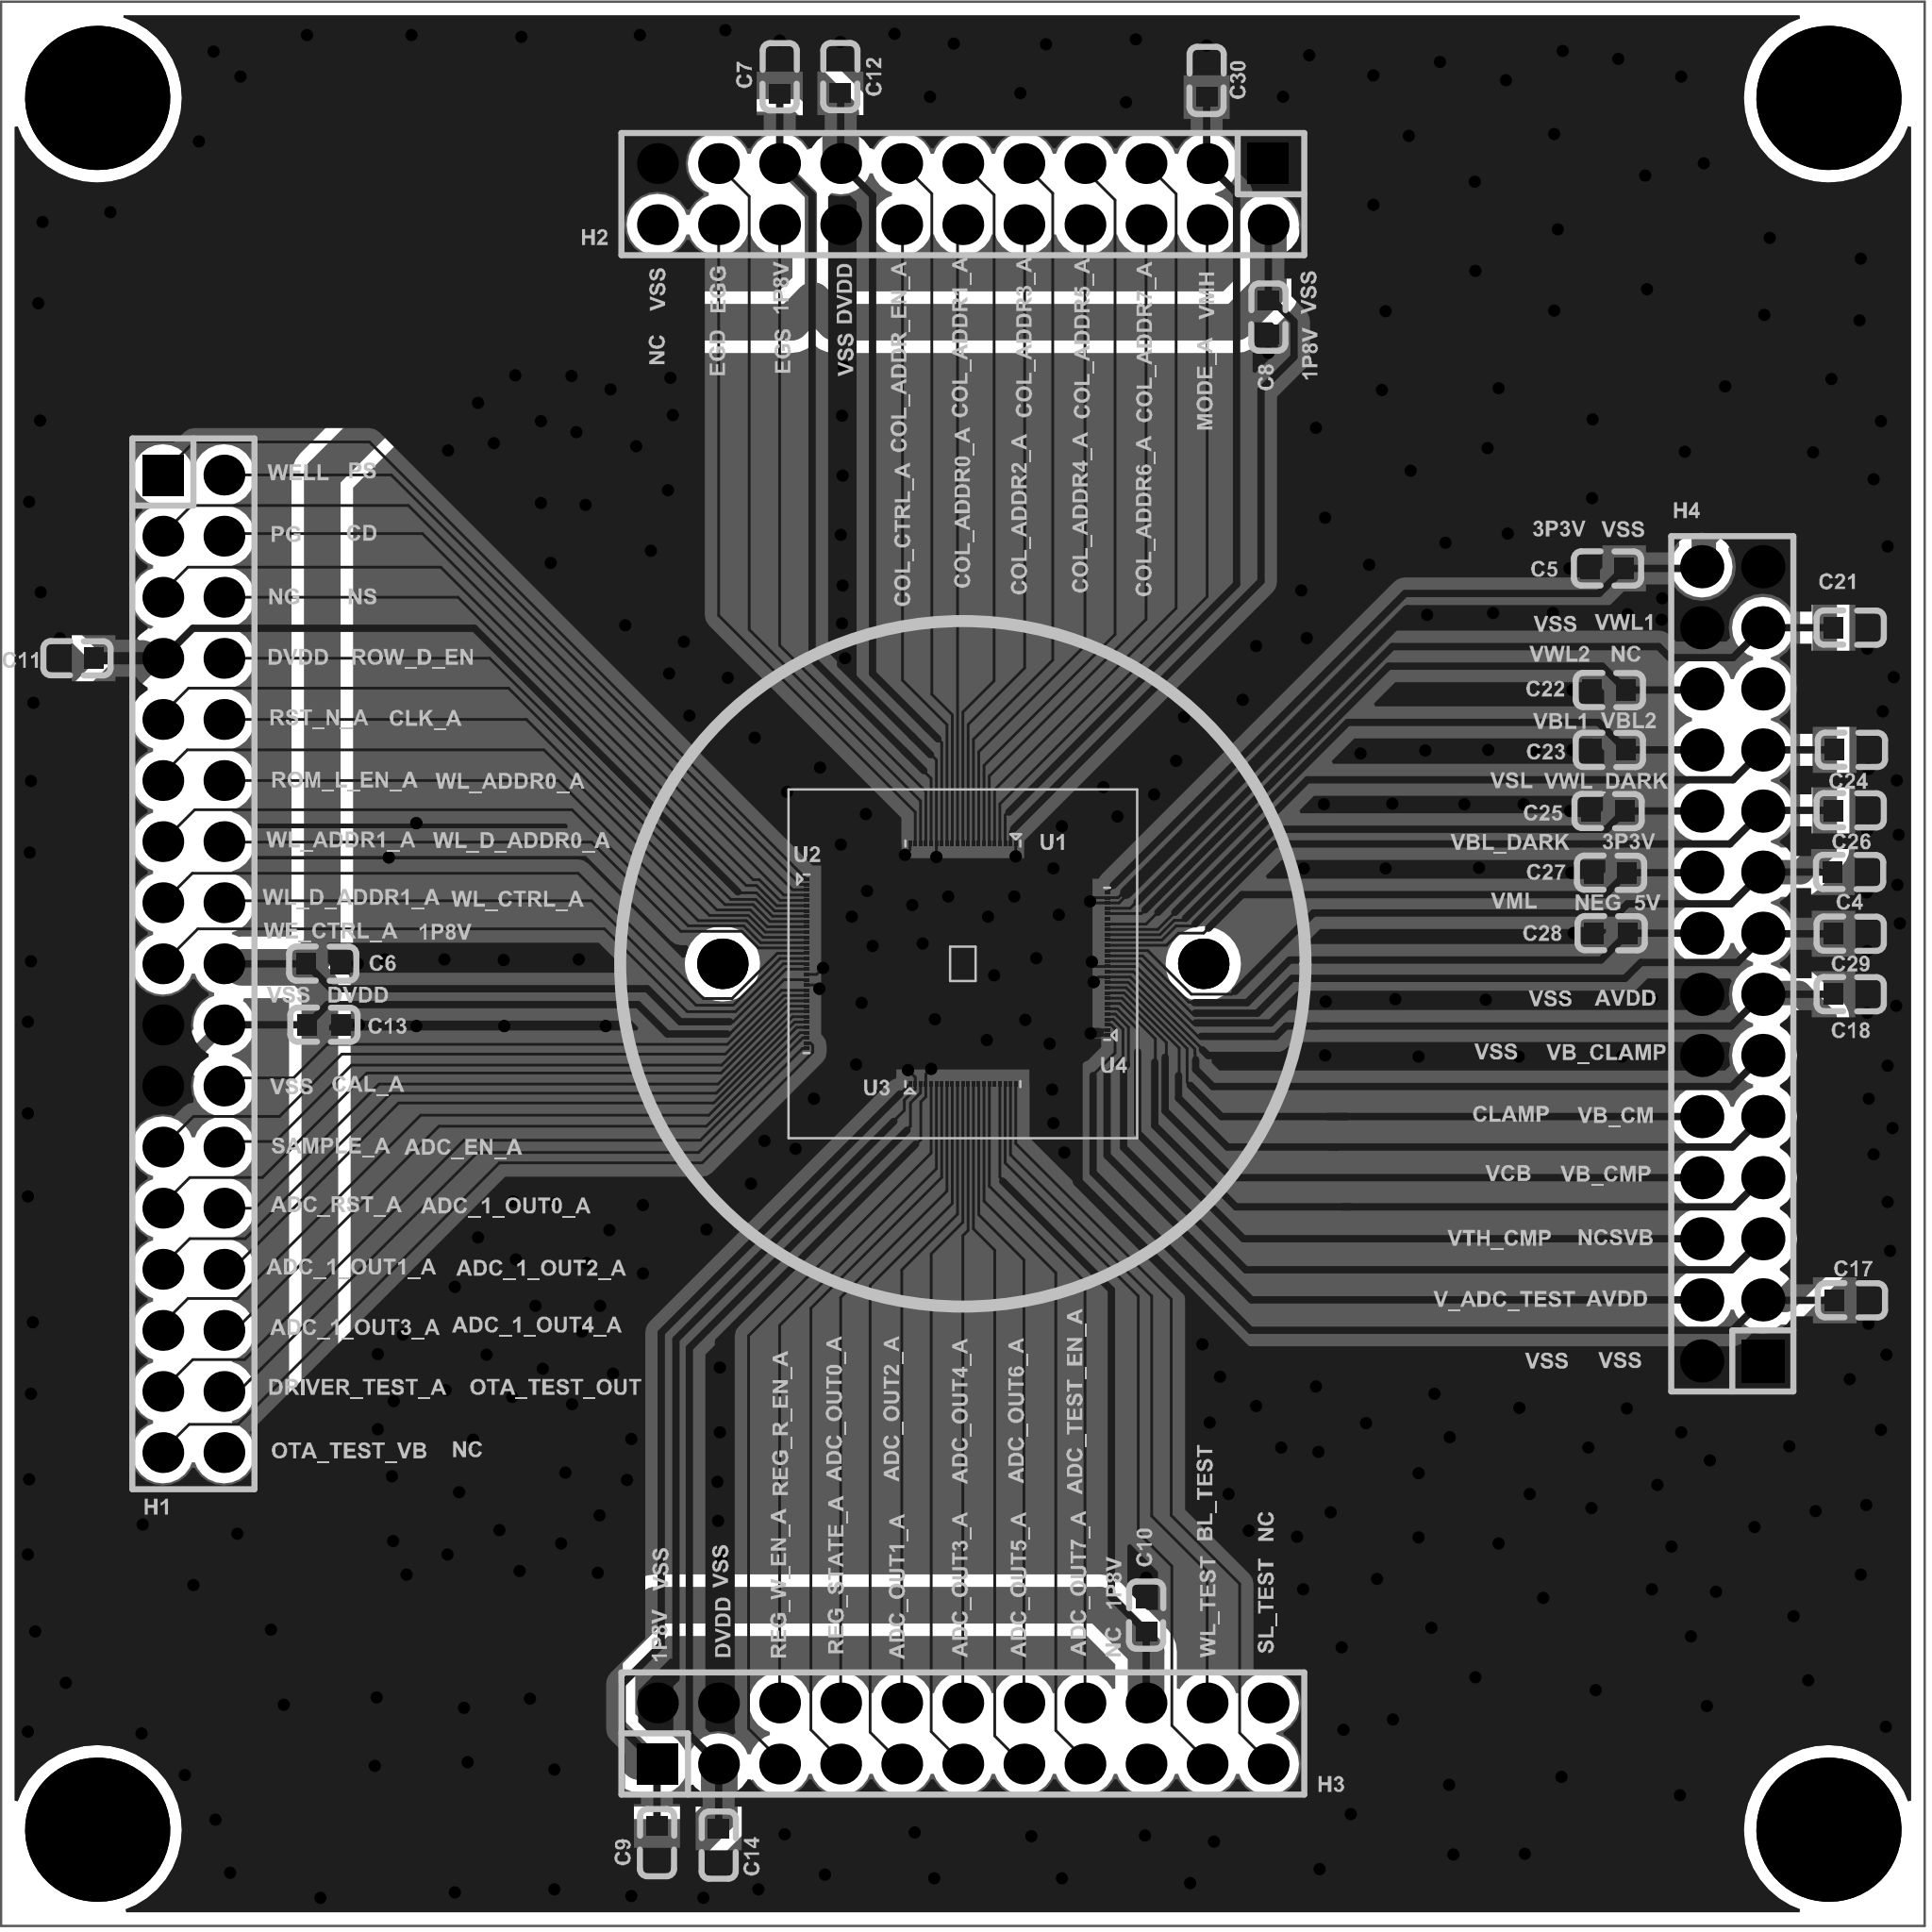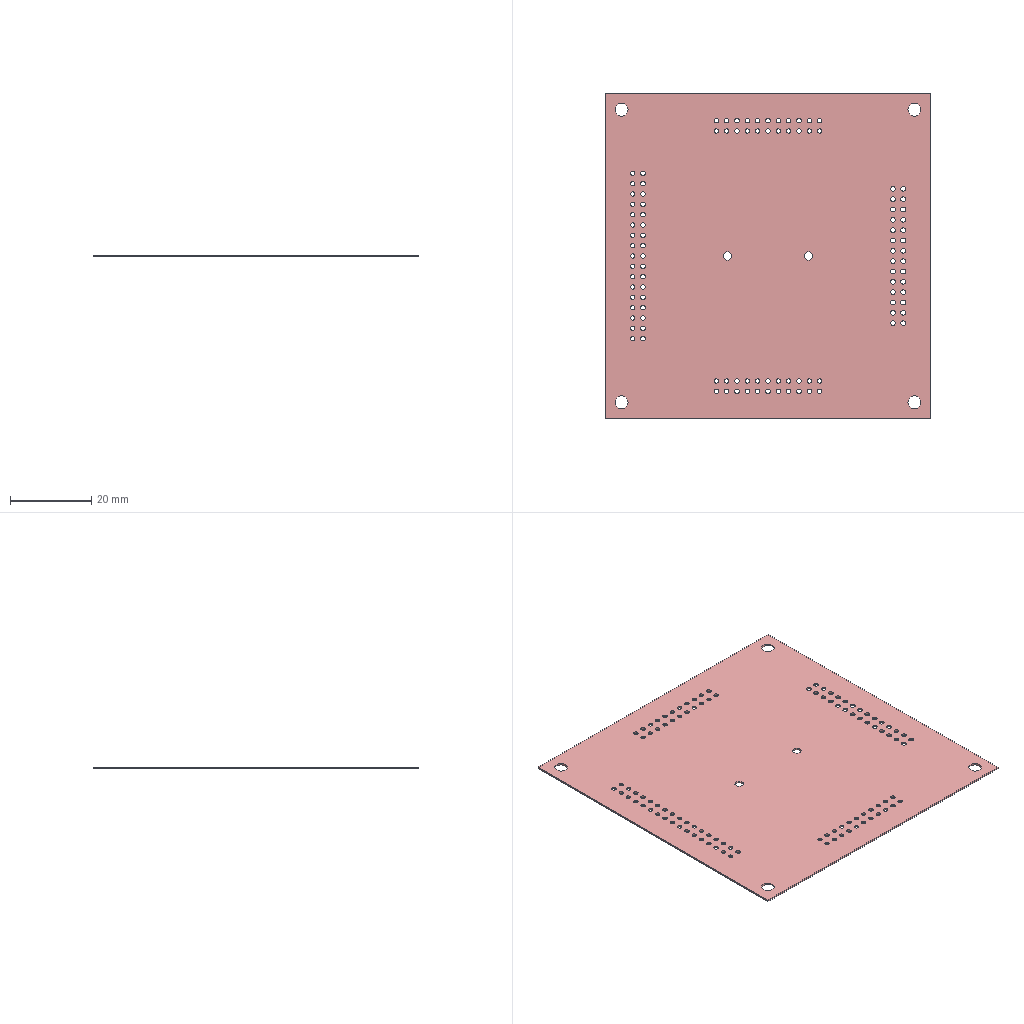Circuit board layout | Altium Designer | box 80 x 80 x 0.4 mm
Layer stack:
# Altium Designer layer stack of  (unit mm; dielectric type: 0 none, 1 core, 2 prepreg, 3 surface material)
index,name,kind,layer,copper_thickness_mm,dielectric_type,dielectric_thickness_mm,dielectric_material,dielectric_constant
0,Top Paste,other,,,,,,
1,Top Overlay,other,,,,,,
2,Top Solder,dielectric,,,3,0.0102,Solder Resist,3.5
3,Top Layer,copper,Top Layer,0.0356,,,,
4,Dielectric1,dielectric,,,0,0.32,FR-4,4.8
5,Bottom Layer,copper,Bottom Layer,0.0356,,,,
6,Bottom Solder,dielectric,,,3,0.0102,Solder Resist,3.5
7,Bottom Overlay,other,,,,,,
8,Bottom Paste,other,,,,,,
# drill layer pairs: low layer,high layer
drill_pair,Top Layer,Bottom Layer
Part placement:
Designator,Comment,Layer,Footprint,Center-X(mm),Center-Y(mm),Rotation
C18,100nF/16V,TopLayer,0603C,76.911,38.735,360
C17,100nF/16V,TopLayer,0603C,76.962,26.01,360
C14,100nF/16V,TopLayer,0603C,29.845,3.353,270
C13,100nF/16V,TopLayer,0603C,13.437,37.465,360
C12,100nF/16V,TopLayer,0603C,34.907,76.893,90
C11,100nF/16V,TopLayer,0603C,3.15,52.705,180
C10,100nF/16V,TopLayer,0603C,47.625,12.929,90
C9,100nF/16V,TopLayer,0603C,27.28,3.454,270
C8,100nF/16V,TopLayer,0603C,52.705,66.878,270
C7,100nF/16V,TopLayer,0603C,32.385,76.886,90
C6,100nF/16V,TopLayer,0603C,13.386,40.005,0
C5,100nF/16V,TopLayer,0603C,66.802,56.439,180
C4,100nF/16V,TopLayer,0603C,76.886,43.815,0
U4,X6511WVS-28H-C60D48R1,TopLayer,JSZ28,46,40,180
U3,X6511WVS-21H-C60D48R2,TopLayer,JSZ21,40,35,90
U2,X6511WVS-33H-C60D48R2,TopLayer,JSZ33,33.5,40,0
U1,X6511WVS-21H-C60D48R2,TopLayer,JSZ21,40,45,270
H4,#NAME?,TopLayer,HDR-TH_28P-P2.54-V-M-R2-C14-S2.54,72,40,90
H3,#NAME?,TopLayer,HDR-TH_22P-P2.54-V-M-R2-C11-S2.54,40,8,360
H2,#NAME?,TopLayer,HDR-TH_22P-P2.54-V-M-R2-C11-S2.54,40,72,180
H1,#NAME?,TopLayer,HDR-TH_34P-P2.54-V-M-R2-C17-S2.54,8,40,270
C21,100nF/16V,TopLayer,0603C,76.911,53.975,0
C22,100nF/16V,TopLayer,0603C,66.878,51.384,180
C23,100nF/16V,TopLayer,0603C,66.878,48.895,180
C24,100nF/16V,TopLayer,0603C,76.962,48.895,360
C25,100nF/16V,TopLayer,0603C,66.827,46.355,180
C26,100nF/16V,TopLayer,0603C,76.911,46.38,360
C27,100nF/16V,TopLayer,0603C,66.929,43.79,180
C28,100nF/16V,TopLayer,0603C,66.954,41.275,180
C29,100nF/16V,TopLayer,0603C,76.911,41.25,360
C30,100nF/16V,TopLayer,0603C,50.14,76.733,90
Pad and via stacks:
# Altium Designer via and pad stacks of  (unit mm). Each distinct definition once, with the count of objects using it.
# via: kind,start_layer,end_layer,hole_mm,diameter_mm,mode(0 simple;1 top-mid-bottom;2 full stack),diameter_per_layer,count,example_net
# pad: kind,layer,hole_mm,hole_type(0 round;1 square;2 slot),plating,top_size,top_shape(1 round;2 rect;3 octagon;9 rounded rect),mid_size,bottom_size,mode,footprint,size_per_layer,count,example
pad,Multi-Layer,2.1,0,unplated,2.1x2.1,1,2.1x2.1,2.1x2.1,0,,,2,0
pad,Multi-Layer,3.2,0,plated,6x6,1,6x6,6x6,0,,,4,2
pad,Multi-Layer,1.1,0,plated,1.7x1.7,1,1.524x1.524,1.524x1.524,1,HDR-TH_22P-P2.54-V-M-R2-C11-S2.54,,41,H2.22
pad,Multi-Layer,1.1,0,plated,1.7x1.7,1,1.7x1.7,1.7x1.7,1,HDR-TH_22P-P2.54-V-M-R2-C11-S2.54,,1,H2.21
pad,Multi-Layer,1.1,0,plated,1.7x1.7,2,1.524x1.524,1.524x1.524,1,HDR-TH_22P-P2.54-V-M-R2-C11-S2.54,,2,H2.1
pad,Multi-Layer,1.1,0,plated,1.7x1.7,2,1.524x1.524,1.524x1.524,1,HDR-TH_34P-P2.54-V-M-R2-C17-S2.54,,1,H1.1
pad,Multi-Layer,1.1,0,plated,1.7x1.7,1,1.524x1.524,1.524x1.524,1,HDR-TH_34P-P2.54-V-M-R2-C17-S2.54,,33,H1.2
pad,Multi-Layer,1.2,0,plated,1.8x1.8,2,1.524x1.524,1.524x1.524,1,HDR-TH_28P-P2.54-V-M-R2-C14-S2.54,,1,H4.1
pad,Multi-Layer,1.2,0,plated,1.8x1.8,1,1.524x1.524,1.524x1.524,1,HDR-TH_28P-P2.54-V-M-R2-C14-S2.54,,27,H4.2
pad,Top Layer,0,0,plated,0.8x0.9,2,0.8x0.9,0.8x0.9,0,0603C,,46,C5.1
pad,Top Layer,0,0,plated,0.12x0.2,2,0.12x0.2,0.12x0.2,0,JSZ21,,42,U1.21
pad,Top Layer,0,0,plated,0.12x0.2,2,0.12x0.2,0.12x0.2,0,JSZ33,,33,U2.33
pad,Top Layer,0,0,plated,0.12x0.2,2,0.12x0.2,0.12x0.2,0,JSZ28,,28,U4.28
via,Top Layer,Bottom Layer,0.3048,0.508,0,,355,VSS
Copper pours:
name,layer,net,type(0 solid;1 hatched;2 none)
Bottom Layer-No Net,Top Layer,VSS,0
Bottom Layer-No Net,Bottom Layer,VSS,0
Design rules, without the lines most boards share:
# Altium Designer design rules of  (exported by Altium Designer, unit mm)
# columns: name | kind | enabled | priority | scope1 | scope2 | descriptor | typed fields (field=value)
Clearance_1 | 0 | enabled | 2 | ispad | ispad | Clearance Constraint (Gap=3mil) (ispad),(ispad) | gap=0.0762
SilkToSilkClearance | 55 | enabled | 1 | All | All | Silk to Silk (Clearance=0mil) (All),(All) |
SilkscreenOverComponentPads | 54 | enabled | 1 | IsPad | All | Silk To Solder Mask (Clearance=0mil) (IsPad),(All) |
MinimumSolderMaskSliver | 53 | enabled | 1 | All | All | Minimum Solder Mask Sliver (Gap=0mil) (All),(All) |
HoleToHoleClearance | 52 | enabled | 1 | All | All | Hole To Hole Clearance (Gap=0mil) (All),(All) | gap=0
DiffPairsRouting | 51 | enabled | 1 | All | All | Differential Pairs Uncoupled Length using the Gap Constraints (Min=10mil) (Max=10mil) (Prefered=10mil)  and Width Constraints (Min=15mil) (Max=15mil) (Prefered=15mil) (All) |
HoleSize | 42 | enabled | 1 | All | All | Hole Size Constraint (Min=1mil) (Max=500mil) (All) |
SolderMaskExpansion | 13 | enabled | 1 | All | All | Solder Mask Expansion (Expansion =4mil) (All) | expansion=0.1016
PasteMaskExpansion | 14 | enabled | 1 | All | All | Paste Mask Expansion (Expansion =0mil) (All) | expansion=0
RoutingVias | 11 | enabled | 1 | All | All | Routing Via (MinHoleWidth=12mil) (MaxHoleWidth=12mil) (PreferredHoleWidth=12mil) (MinWidth=20mil) (MaxWidth=20mil) (PreferedWidth=20mil) (All) | via_min_hole=0.3048 via_max_hole=0.3048 via_preferred_diameter=0.508 via_preferred_hole=0.3048
Width | 2 | enabled | 1 | All | All | Width Constraint (Min=4mil) (Max=80mil) (Preferred=4mil) (All) |
PolygonConnect | 20 | enabled | 1 | All | All | Polygon Connect Rule(Direct Connect )(Conductor Width=10mil) (Relief Angle=90 Angle) (Entries=4) (Air Gap Width=10mil) (All),(All) | connect_style(0=relief,1=direct,2=none)=1 relief_conductor_width=0.254 relief_entries=4
PlaneClearance | 12 | enabled | 1 | All | All | Power Plane Clearance (Clearance =6mil) (All) | clearance=0.1524
PlaneConnect | 6 | enabled | 1 | All | All | Power Plane Connect Rule(Direct Connect )(Expansion=20mil) (Conductor Width=10mil) (Air Gap=10mil) (Entries=4) (All) | relief_conductor_width=0.254 relief_entries=4 relief_expansion=0.508
Clearance | 0 | enabled | 3 | All | All | Clearance Constraint (Gap=4mil) (All),(All) | gap=0.1016
Clearance_2 | 0 | enabled | 1 | inpolygon | All | Clearance Constraint (Gap=20mil) (inpolygon),(All) | gap=0.508
Classes set for this board:
# Altium Designer classes of  (member kind: 0 net, 1 component, 2 from-to, 3 pad, 4 layer, 5 differential pair, 6 design channel, 7 polygon, 8 structure, 9 xSignal)
# columns: class name | member kind | superclass | members
1_YHZ_COB.schdoc | 1 | no | H1; H2; H3; H4; U1; U2; U3; U4; C4; C5; C6; C7; C8; C9; C10; C11; C12; C13; C14; C17; C18; C21; C22; C23; C24; C25; C26; C27; C28; C29; C30;